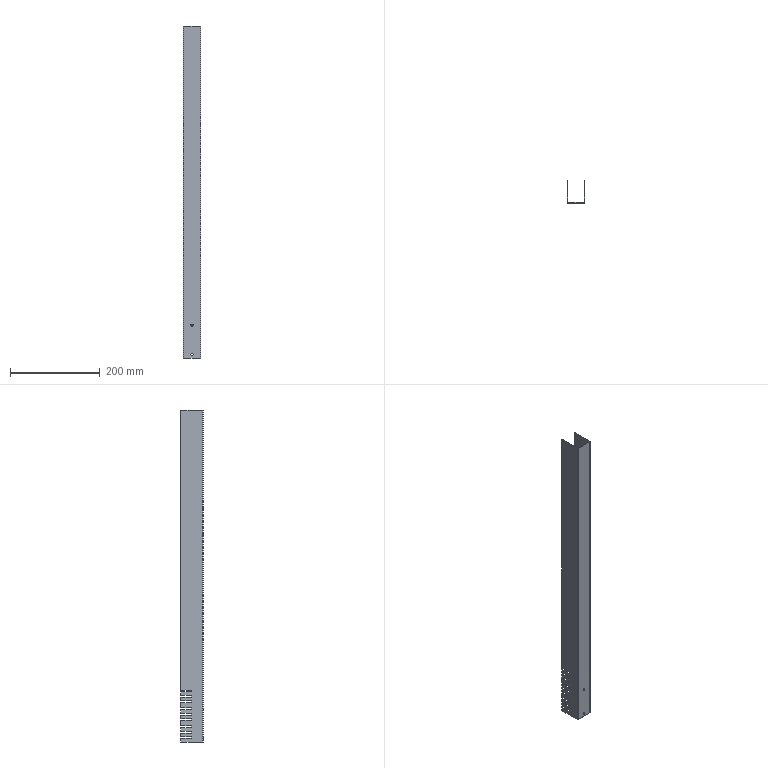Part | SolidWorks | features Cut 1, FlatPattern 1, ICE 1, LPattern 1, SMBaseFlange 1, SheetMetal 1 | 1 solid | 98 faces | box 40 x 50 x 741 mm | volume 148783 mm3 | plane 90 | cylinder 8 | commonest cylinder face diameters 5 x4 0.4 x2 3.4 x2